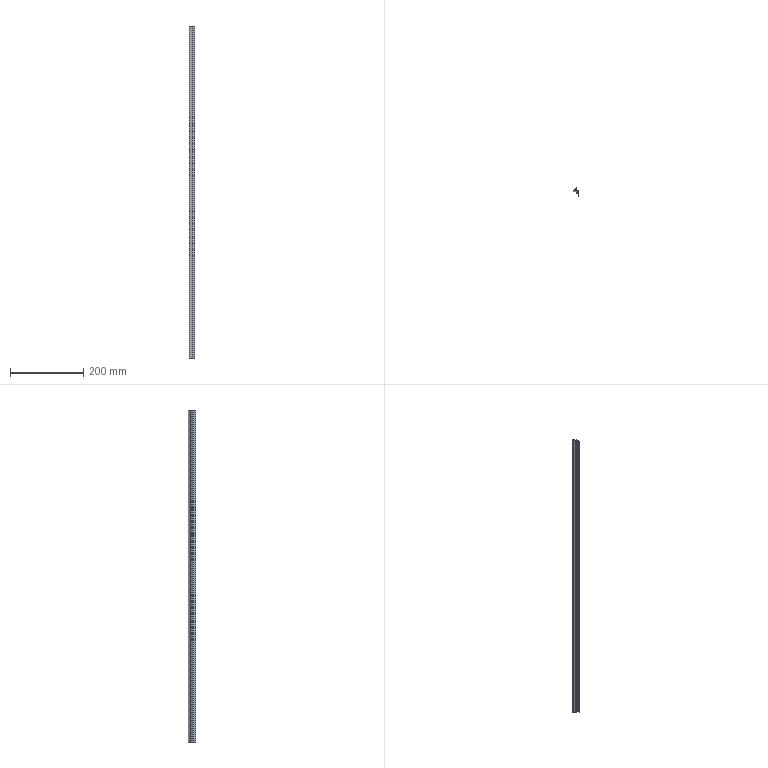Part | SolidWorks | features BaseBody 1, ICE 1, MoveFace 1 | 1 solid | 27 faces | box 14 x 20.3 x 907 mm | volume 46181 mm3 | plane 20 | cylinder 7 | commonest cylinder face diameters 0.387 x2 0.8 x2 0.4 x1 20 x1 22 x1
STEP:
#1=CARTESIAN_POINT('',(-5.304,-0.625,200.));
#2=VERTEX_POINT('',#1);
#3=CARTESIAN_POINT('',(-5.449,-0.8125,200.));
#4=VERTEX_POINT('',#3);
#5=CARTESIAN_POINT('',(-5.255,-0.8125,200.));
#6=DIRECTION('',(0.,0.,1.));
#7=DIRECTION('',(-1.,0.,0.));
#8=AXIS2_PLACEMENT_3D('',#5,#6,#7);
#9=CIRCLE('',#8,0.1937);
#10=EDGE_CURVE('',#2,#4,#9,.T.);
#11=ORIENTED_EDGE('',*,*,#10,.T.);
#12=CARTESIAN_POINT('',(-5.449,-0.8125,-707.));
#13=VERTEX_POINT('',#12);
#14=CARTESIAN_POINT('',(-5.449,-0.8125,230.));
#15=DIRECTION('',(0.,0.,-1.));
#16=VECTOR('',#15,1000.);
#17=LINE('',#14,#16);
#18=EDGE_CURVE('',#4,#13,#17,.T.);
#19=ORIENTED_EDGE('',*,*,#18,.T.);
#20=CARTESIAN_POINT('',(-5.304,-0.625,-707.));
#21=VERTEX_POINT('',#20);
#22=CARTESIAN_POINT('',(-5.255,-0.8125,-707.));
#23=DIRECTION('',(0.,0.,-1.));
#24=DIRECTION('',(1.,0.,0.));
#25=AXIS2_PLACEMENT_3D('',#22,#23,#24);
#26=CIRCLE('',#25,0.1937);
#27=EDGE_CURVE('',#13,#21,#26,.T.);
#28=ORIENTED_EDGE('',*,*,#27,.T.);
#29=CARTESIAN_POINT('',(-5.304,-0.625,230.));
#30=DIRECTION('',(0.,0.,-1.));
#31=VECTOR('',#30,1000.);
#32=LINE('',#29,#31);
#33=EDGE_CURVE('',#2,#21,#32,.T.);
#34=ORIENTED_EDGE('',*,*,#33,.F.);
#35=EDGE_LOOP('',(#11,#19,#28,#34));
#36=FACE_OUTER_BOUND('',#35,.T.);
#37=CARTESIAN_POINT('',(-5.255,-0.8125,230.));
#38=DIRECTION('',(0.,0.,-1.));
#39=DIRECTION('',(-1.,0.,0.));
#40=AXIS2_PLACEMENT_3D('',#37,#38,#39);
#41=CYLINDRICAL_SURFACE('',#40,0.1937);
#42=ADVANCED_FACE('',(#36),#41,.F.);
#43=CARTESIAN_POINT('',(5.,-1.,-707.));
#44=VERTEX_POINT('',#43);
#45=CARTESIAN_POINT('',(5.,-14.3,-707.));
#46=VERTEX_POINT('',#45);
#47=CARTESIAN_POINT('',(5.,29.623,-707.));
#48=DIRECTION('',(0.,-1.,0.));
#49=VECTOR('',#48,1000.);
#50=LINE('',#47,#49);
#51=EDGE_CURVE('',#44,#46,#50,.T.);
#52=ORIENTED_EDGE('',*,*,#51,.F.);
#53=CARTESIAN_POINT('',(5.,-1.,200.));
#54=VERTEX_POINT('',#53);
#55=CARTESIAN_POINT('',(5.,-1.,230.));
#56=DIRECTION('',(0.,0.,-1.));
#57=VECTOR('',#56,1000.);
#58=LINE('',#55,#57);
#59=EDGE_CURVE('',#54,#44,#58,.T.);
#60=ORIENTED_EDGE('',*,*,#59,.F.);
#61=CARTESIAN_POINT('',(5.,-14.3,200.));
#62=VERTEX_POINT('',#61);
#63=CARTESIAN_POINT('',(5.,-14.3,200.));
#64=DIRECTION('',(0.,1.,0.));
#65=VECTOR('',#64,1000.);
#66=LINE('',#63,#65);
#67=EDGE_CURVE('',#62,#54,#66,.T.);
#68=ORIENTED_EDGE('',*,*,#67,.F.);
#69=CARTESIAN_POINT('',(5.,-14.3,230.));
#70=DIRECTION('',(0.,0.,1.));
#71=VECTOR('',#70,1000.);
#72=LINE('',#69,#71);
#73=EDGE_CURVE('',#46,#62,#72,.T.);
#74=ORIENTED_EDGE('',*,*,#73,.F.);
#75=EDGE_LOOP('',(#52,#60,#68,#74));
#76=FACE_OUTER_BOUND('',#75,.T.);
#77=CARTESIAN_POINT('',(5.,-14.3,230.));
#78=DIRECTION('',(-1.,0.,0.));
#79=DIRECTION('',(0.,0.,1.));
#80=AXIS2_PLACEMENT_3D('',#77,#78,#79);
#81=PLANE('',#80);
#82=ADVANCED_FACE('',(#76),#81,.F.);
#83=CARTESIAN_POINT('',(-9.,-2.,-707.));
#84=VERTEX_POINT('',#83);
#85=CARTESIAN_POINT('',(-9.,-2.,200.));
#86=VERTEX_POINT('',#85);
#87=CARTESIAN_POINT('',(-9.,-2.,230.));
#88=DIRECTION('',(0.,0.,1.));
#89=VECTOR('',#88,1000.);
#90=LINE('',#87,#89);
#91=EDGE_CURVE('',#84,#86,#90,.T.);
#92=ORIENTED_EDGE('',*,*,#91,.F.);
#93=CARTESIAN_POINT('',(0.9,-2.,-707.));
#94=VERTEX_POINT('',#93);
#95=CARTESIAN_POINT('',(5.,-2.,-707.));
#96=DIRECTION('',(-1.,0.,0.));
#97=VECTOR('',#96,1000.);
#98=LINE('',#95,#97);
#99=EDGE_CURVE('',#94,#84,#98,.T.);
#100=ORIENTED_EDGE('',*,*,#99,.F.);
#101=CARTESIAN_POINT('',(0.9,-2.,200.));
#102=VERTEX_POINT('',#101);
#103=CARTESIAN_POINT('',(0.9,-2.,230.));
#104=DIRECTION('',(0.,0.,-1.));
#105=VECTOR('',#104,1000.);
#106=LINE('',#103,#105);
#107=EDGE_CURVE('',#102,#94,#106,.T.);
#108=ORIENTED_EDGE('',*,*,#107,.F.);
#109=CARTESIAN_POINT('',(5.,-2.,200.));
#110=DIRECTION('',(1.,0.,0.));
#111=VECTOR('',#110,1000.);
#112=LINE('',#109,#111);
#113=EDGE_CURVE('',#86,#102,#112,.T.);
#114=ORIENTED_EDGE('',*,*,#113,.F.);
#115=EDGE_LOOP('',(#92,#100,#108,#114));
#116=FACE_OUTER_BOUND('',#115,.T.);
#117=CARTESIAN_POINT('',(-9.,-2.,230.));
#118=DIRECTION('',(0.,1.,0.));
#119=DIRECTION('',(0.,0.,1.));
#120=AXIS2_PLACEMENT_3D('',#117,#118,#119);
#121=PLANE('',#120);
#122=ADVANCED_FACE('',(#116),#121,.F.);
#123=CARTESIAN_POINT('',(4.,-6.,200.));
#124=VERTEX_POINT('',#123);
#125=CARTESIAN_POINT('',(4.,-3.,200.));
#126=VERTEX_POINT('',#125);
#127=CARTESIAN_POINT('',(4.,29.623,200.));
#128=DIRECTION('',(0.,1.,0.));
#129=VECTOR('',#128,1000.);
#130=LINE('',#127,#129);
#131=EDGE_CURVE('',#124,#126,#130,.T.);
#132=ORIENTED_EDGE('',*,*,#131,.F.);
#133=CARTESIAN_POINT('',(1.,-6.,200.));
#134=VERTEX_POINT('',#133);
#135=CARTESIAN_POINT('',(5.,-6.,200.));
#136=DIRECTION('',(1.,0.,0.));
#137=VECTOR('',#136,1000.);
#138=LINE('',#135,#137);
#139=EDGE_CURVE('',#134,#124,#138,.T.);
#140=ORIENTED_EDGE('',*,*,#139,.F.);
#141=CARTESIAN_POINT('',(1.,-6.7,200.));
#142=VERTEX_POINT('',#141);
#143=CARTESIAN_POINT('',(1.,-6.,200.));
#144=DIRECTION('',(0.,-1.,0.));
#145=VECTOR('',#144,1000.);
#146=LINE('',#143,#145);
#147=EDGE_CURVE('',#134,#142,#146,.T.);
#148=ORIENTED_EDGE('',*,*,#147,.T.);
#149=CARTESIAN_POINT('',(-1.7,-6.7,200.));
#150=VERTEX_POINT('',#149);
#151=CARTESIAN_POINT('',(5.,-6.7,200.));
#152=DIRECTION('',(1.,0.,0.));
#153=VECTOR('',#152,1000.);
#154=LINE('',#151,#153);
#155=EDGE_CURVE('',#150,#142,#154,.T.);
#156=ORIENTED_EDGE('',*,*,#155,.F.);
#157=CARTESIAN_POINT('',(-1.7,-7.7,200.));
#158=VERTEX_POINT('',#157);
#159=CARTESIAN_POINT('',(-1.7,-6.7,200.));
#160=DIRECTION('',(0.,-1.,0.));
#161=VECTOR('',#160,1000.);
#162=LINE('',#159,#161);
#163=EDGE_CURVE('',#150,#158,#162,.T.);
#164=ORIENTED_EDGE('',*,*,#163,.T.);
#165=CARTESIAN_POINT('',(4.,-7.7,200.));
#166=VERTEX_POINT('',#165);
#167=CARTESIAN_POINT('',(5.,-7.7,200.));
#168=DIRECTION('',(-1.,0.,0.));
#169=VECTOR('',#168,1000.);
#170=LINE('',#167,#169);
#171=EDGE_CURVE('',#166,#158,#170,.T.);
#172=ORIENTED_EDGE('',*,*,#171,.F.);
#173=CARTESIAN_POINT('',(4.,-14.3,200.));
#174=VERTEX_POINT('',#173);
#175=CARTESIAN_POINT('',(4.,29.623,200.));
#176=DIRECTION('',(0.,1.,0.));
#177=VECTOR('',#176,1000.);
#178=LINE('',#175,#177);
#179=EDGE_CURVE('',#174,#166,#178,.T.);
#180=ORIENTED_EDGE('',*,*,#179,.F.);
#181=CARTESIAN_POINT('',(5.,-14.3,200.));
#182=DIRECTION('',(-1.,0.,0.));
#183=VECTOR('',#182,1000.);
#184=LINE('',#181,#183);
#185=EDGE_CURVE('',#62,#174,#184,.T.);
#186=ORIENTED_EDGE('',*,*,#185,.F.);
#187=ORIENTED_EDGE('',*,*,#67,.T.);
#188=CARTESIAN_POINT('',(-5.207,-1.,200.));
#189=VERTEX_POINT('',#188);
#190=CARTESIAN_POINT('',(5.,-1.,200.));
#191=DIRECTION('',(1.,0.,0.));
#192=VECTOR('',#191,1000.);
#193=LINE('',#190,#192);
#194=EDGE_CURVE('',#189,#54,#193,.T.);
#195=ORIENTED_EDGE('',*,*,#194,.F.);
#196=CARTESIAN_POINT('',(-5.255,-0.8125,200.));
#197=DIRECTION('',(0.,0.,1.));
#198=DIRECTION('',(-1.,0.,0.));
#199=AXIS2_PLACEMENT_3D('',#196,#197,#198);
#200=CIRCLE('',#199,0.1937);
#201=EDGE_CURVE('',#4,#189,#200,.T.);
#202=ORIENTED_EDGE('',*,*,#201,.F.);
#203=ORIENTED_EDGE('',*,*,#10,.F.);
#204=CARTESIAN_POINT('',(-1.368,3.063,200.));
#205=VERTEX_POINT('',#204);
#206=CARTESIAN_POINT('',(-10.628,9.,200.));
#207=DIRECTION('',(0.,0.,1.));
#208=DIRECTION('',(-1.,0.,0.));
#209=AXIS2_PLACEMENT_3D('',#206,#207,#208);
#210=CIRCLE('',#209,11.);
#211=EDGE_CURVE('',#2,#205,#210,.T.);
#212=ORIENTED_EDGE('',*,*,#211,.T.);
#213=CARTESIAN_POINT('',(-1.,2.955,200.));
#214=VERTEX_POINT('',#213);
#215=CARTESIAN_POINT('',(-1.2,2.955,200.));
#216=DIRECTION('',(0.,0.,1.));
#217=DIRECTION('',(-1.,0.,0.));
#218=AXIS2_PLACEMENT_3D('',#215,#216,#217);
#219=CIRCLE('',#218,0.2);
#220=EDGE_CURVE('',#214,#205,#219,.T.);
#221=ORIENTED_EDGE('',*,*,#220,.F.);
#222=CARTESIAN_POINT('',(-1.,1.5,200.));
#223=VERTEX_POINT('',#222);
#224=CARTESIAN_POINT('',(-1.,2.955,200.));
#225=DIRECTION('',(0.,1.,0.));
#226=VECTOR('',#225,1000.);
#227=LINE('',#224,#226);
#228=EDGE_CURVE('',#223,#214,#227,.T.);
#229=ORIENTED_EDGE('',*,*,#228,.F.);
#230=CARTESIAN_POINT('',(0.,1.5,200.));
#231=VERTEX_POINT('',#230);
#232=CARTESIAN_POINT('',(-1.,1.5,200.));
#233=DIRECTION('',(-1.,0.,0.));
#234=VECTOR('',#233,1000.);
#235=LINE('',#232,#234);
#236=EDGE_CURVE('',#231,#223,#235,.T.);
#237=ORIENTED_EDGE('',*,*,#236,.F.);
#238=CARTESIAN_POINT('',(0.,6.,200.));
#239=VERTEX_POINT('',#238);
#240=CARTESIAN_POINT('',(0.,1.5,200.));
#241=DIRECTION('',(0.,-1.,0.));
#242=VECTOR('',#241,1000.);
#243=LINE('',#240,#242);
#244=EDGE_CURVE('',#239,#231,#243,.T.);
#245=ORIENTED_EDGE('',*,*,#244,.F.);
#246=CARTESIAN_POINT('',(-0.8,6.,200.));
#247=VERTEX_POINT('',#246);
#248=CARTESIAN_POINT('',(0.,6.,200.));
#249=DIRECTION('',(1.,0.,0.));
#250=VECTOR('',#249,1000.);
#251=LINE('',#248,#250);
#252=EDGE_CURVE('',#247,#239,#251,.T.);
#253=ORIENTED_EDGE('',*,*,#252,.F.);
#254=CARTESIAN_POINT('',(-1.178,5.731,200.));
#255=VERTEX_POINT('',#254);
#256=CARTESIAN_POINT('',(-0.8,5.6,200.));
#257=DIRECTION('',(0.,0.,1.));
#258=DIRECTION('',(-1.,0.,0.));
#259=AXIS2_PLACEMENT_3D('',#256,#257,#258);
#260=CIRCLE('',#259,0.4);
#261=EDGE_CURVE('',#247,#255,#260,.T.);
#262=ORIENTED_EDGE('',*,*,#261,.T.);
#263=CARTESIAN_POINT('',(-8.678,-0.8077,200.));
#264=VERTEX_POINT('',#263);
#265=CARTESIAN_POINT('',(-10.628,9.,200.));
#266=DIRECTION('',(0.,0.,1.));
#267=DIRECTION('',(-1.,0.,0.));
#268=AXIS2_PLACEMENT_3D('',#265,#266,#267);
#269=CIRCLE('',#268,10.);
#270=EDGE_CURVE('',#264,#255,#269,.T.);
#271=ORIENTED_EDGE('',*,*,#270,.F.);
#272=CARTESIAN_POINT('',(-9.,-1.2,200.));
#273=VERTEX_POINT('',#272);
#274=CARTESIAN_POINT('',(-8.6,-1.2,200.));
#275=DIRECTION('',(0.,0.,1.));
#276=DIRECTION('',(-1.,0.,0.));
#277=AXIS2_PLACEMENT_3D('',#274,#275,#276);
#278=CIRCLE('',#277,0.4);
#279=EDGE_CURVE('',#264,#273,#278,.T.);
#280=ORIENTED_EDGE('',*,*,#279,.T.);
#281=CARTESIAN_POINT('',(-9.,8.,200.));
#282=DIRECTION('',(0.,-1.,0.));
#283=VECTOR('',#282,1000.);
#284=LINE('',#281,#283);
#285=EDGE_CURVE('',#273,#86,#284,.T.);
#286=ORIENTED_EDGE('',*,*,#285,.T.);
#287=ORIENTED_EDGE('',*,*,#113,.T.);
#288=CARTESIAN_POINT('',(0.9,-3.,200.));
#289=VERTEX_POINT('',#288);
#290=CARTESIAN_POINT('',(0.9,29.623,200.));
#291=DIRECTION('',(0.,1.,0.));
#292=VECTOR('',#291,1000.);
#293=LINE('',#290,#292);
#294=EDGE_CURVE('',#289,#102,#293,.T.);
#295=ORIENTED_EDGE('',*,*,#294,.F.);
#296=CARTESIAN_POINT('',(5.,-3.,200.));
#297=DIRECTION('',(-1.,0.,0.));
#298=VECTOR('',#297,1000.);
#299=LINE('',#296,#298);
#300=EDGE_CURVE('',#126,#289,#299,.T.);
#301=ORIENTED_EDGE('',*,*,#300,.F.);
#302=EDGE_LOOP('',(#132,#140,#148,#156,#164,#172,#180,#186,#187,#195,#202,#203,#212,#221,#229,#237,#245,#253,#262,#271,#280,#286,#287,#295,#301));
#303=FACE_OUTER_BOUND('',#302,.T.);
#304=CARTESIAN_POINT('',(5.,29.623,200.));
#305=DIRECTION('',(0.,0.,-1.));
#306=DIRECTION('',(-1.,0.,0.));
#307=AXIS2_PLACEMENT_3D('',#304,#305,#306);
#308=PLANE('',#307);
#309=ADVANCED_FACE('',(#303),#308,.F.);
#310=ORIENTED_EDGE('',*,*,#185,.T.);
#311=CARTESIAN_POINT('',(4.,-14.3,-707.));
#312=VERTEX_POINT('',#311);
#313=CARTESIAN_POINT('',(4.,-14.3,230.));
#314=DIRECTION('',(0.,0.,1.));
#315=VECTOR('',#314,1000.);
#316=LINE('',#313,#315);
#317=EDGE_CURVE('',#312,#174,#316,.T.);
#318=ORIENTED_EDGE('',*,*,#317,.F.);
#319=CARTESIAN_POINT('',(5.,-14.3,-707.));
#320=DIRECTION('',(-1.,0.,0.));
#321=VECTOR('',#320,1000.);
#322=LINE('',#319,#321);
#323=EDGE_CURVE('',#46,#312,#322,.T.);
#324=ORIENTED_EDGE('',*,*,#323,.F.);
#325=ORIENTED_EDGE('',*,*,#73,.T.);
#326=EDGE_LOOP('',(#310,#318,#324,#325));
#327=FACE_OUTER_BOUND('',#326,.T.);
#328=CARTESIAN_POINT('',(4.,-14.3,230.));
#329=DIRECTION('',(0.,1.,0.));
#330=DIRECTION('',(0.,0.,1.));
#331=AXIS2_PLACEMENT_3D('',#328,#329,#330);
#332=PLANE('',#331);
#333=ADVANCED_FACE('',(#327),#332,.F.);
#334=ORIENTED_EDGE('',*,*,#51,.T.);
#335=ORIENTED_EDGE('',*,*,#323,.T.);
#336=CARTESIAN_POINT('',(4.,-7.7,-707.));
#337=VERTEX_POINT('',#336);
#338=CARTESIAN_POINT('',(4.,-7.7,-707.));
#339=DIRECTION('',(0.,-1.,0.));
#340=VECTOR('',#339,1000.);
#341=LINE('',#338,#340);
#342=EDGE_CURVE('',#337,#312,#341,.T.);
#343=ORIENTED_EDGE('',*,*,#342,.F.);
#344=CARTESIAN_POINT('',(-1.7,-7.7,-707.));
#345=VERTEX_POINT('',#344);
#346=CARTESIAN_POINT('',(-1.7,-7.7,-707.));
#347=DIRECTION('',(1.,0.,0.));
#348=VECTOR('',#347,1000.);
#349=LINE('',#346,#348);
#350=EDGE_CURVE('',#345,#337,#349,.T.);
#351=ORIENTED_EDGE('',*,*,#350,.F.);
#352=CARTESIAN_POINT('',(-1.7,-6.7,-707.));
#353=VERTEX_POINT('',#352);
#354=CARTESIAN_POINT('',(-1.7,29.623,-707.));
#355=DIRECTION('',(0.,1.,0.));
#356=VECTOR('',#355,1000.);
#357=LINE('',#354,#356);
#358=EDGE_CURVE('',#345,#353,#357,.T.);
#359=ORIENTED_EDGE('',*,*,#358,.T.);
#360=CARTESIAN_POINT('',(1.,-6.7,-707.));
#361=VERTEX_POINT('',#360);
#362=CARTESIAN_POINT('',(1.,-6.7,-707.));
#363=DIRECTION('',(-1.,0.,0.));
#364=VECTOR('',#363,1000.);
#365=LINE('',#362,#364);
#366=EDGE_CURVE('',#361,#353,#365,.T.);
#367=ORIENTED_EDGE('',*,*,#366,.F.);
#368=CARTESIAN_POINT('',(1.,-6.,-707.));
#369=VERTEX_POINT('',#368);
#370=CARTESIAN_POINT('',(1.,29.623,-707.));
#371=DIRECTION('',(0.,1.,0.));
#372=VECTOR('',#371,1000.);
#373=LINE('',#370,#372);
#374=EDGE_CURVE('',#361,#369,#373,.T.);
#375=ORIENTED_EDGE('',*,*,#374,.T.);
#376=CARTESIAN_POINT('',(4.,-6.,-707.));
#377=VERTEX_POINT('',#376);
#378=CARTESIAN_POINT('',(4.,-6.,-707.));
#379=DIRECTION('',(-1.,0.,0.));
#380=VECTOR('',#379,1000.);
#381=LINE('',#378,#380);
#382=EDGE_CURVE('',#377,#369,#381,.T.);
#383=ORIENTED_EDGE('',*,*,#382,.F.);
#384=CARTESIAN_POINT('',(4.,-3.,-707.));
#385=VERTEX_POINT('',#384);
#386=CARTESIAN_POINT('',(4.,-3.,-707.));
#387=DIRECTION('',(0.,-1.,0.));
#388=VECTOR('',#387,1000.);
#389=LINE('',#386,#388);
#390=EDGE_CURVE('',#385,#377,#389,.T.);
#391=ORIENTED_EDGE('',*,*,#390,.F.);
#392=CARTESIAN_POINT('',(0.9,-3.,-707.));
#393=VERTEX_POINT('',#392);
#394=CARTESIAN_POINT('',(0.9,-3.,-707.));
#395=DIRECTION('',(1.,0.,0.));
#396=VECTOR('',#395,1000.);
#397=LINE('',#394,#396);
#398=EDGE_CURVE('',#393,#385,#397,.T.);
#399=ORIENTED_EDGE('',*,*,#398,.F.);
#400=CARTESIAN_POINT('',(0.9,-2.,-707.));
#401=DIRECTION('',(0.,-1.,0.));
#402=VECTOR('',#401,1000.);
#403=LINE('',#400,#402);
#404=EDGE_CURVE('',#94,#393,#403,.T.);
#405=ORIENTED_EDGE('',*,*,#404,.F.);
#406=ORIENTED_EDGE('',*,*,#99,.T.);
#407=CARTESIAN_POINT('',(-9.,-1.2,-707.));
#408=VERTEX_POINT('',#407);
#409=CARTESIAN_POINT('',(-9.,-1.2,-707.));
#410=DIRECTION('',(0.,-1.,0.));
#411=VECTOR('',#410,1000.);
#412=LINE('',#409,#411);
#413=EDGE_CURVE('',#408,#84,#412,.T.);
#414=ORIENTED_EDGE('',*,*,#413,.F.);
#415=CARTESIAN_POINT('',(-8.678,-0.8077,-707.));
#416=VERTEX_POINT('',#415);
#417=CARTESIAN_POINT('',(-8.6,-1.2,-707.));
#418=DIRECTION('',(0.,0.,-1.));
#419=DIRECTION('',(1.,0.,0.));
#420=AXIS2_PLACEMENT_3D('',#417,#418,#419);
#421=CIRCLE('',#420,0.4);
#422=EDGE_CURVE('',#408,#416,#421,.T.);
#423=ORIENTED_EDGE('',*,*,#422,.T.);
#424=CARTESIAN_POINT('',(-1.178,5.731,-707.));
#425=VERTEX_POINT('',#424);
#426=CARTESIAN_POINT('',(-10.628,9.,-707.));
#427=DIRECTION('',(0.,0.,-1.));
#428=DIRECTION('',(1.,0.,0.));
#429=AXIS2_PLACEMENT_3D('',#426,#427,#428);
#430=CIRCLE('',#429,10.);
#431=EDGE_CURVE('',#425,#416,#430,.T.);
#432=ORIENTED_EDGE('',*,*,#431,.F.);
#433=CARTESIAN_POINT('',(-0.8,6.,-707.));
#434=VERTEX_POINT('',#433);
#435=CARTESIAN_POINT('',(-0.8,5.6,-707.));
#436=DIRECTION('',(0.,0.,-1.));
#437=DIRECTION('',(1.,0.,0.));
#438=AXIS2_PLACEMENT_3D('',#435,#436,#437);
#439=CIRCLE('',#438,0.4);
#440=EDGE_CURVE('',#425,#434,#439,.T.);
#441=ORIENTED_EDGE('',*,*,#440,.T.);
#442=CARTESIAN_POINT('',(0.,6.,-707.));
#443=VERTEX_POINT('',#442);
#444=CARTESIAN_POINT('',(0.,6.,-707.));
#445=DIRECTION('',(-1.,0.,0.));
#446=VECTOR('',#445,1000.);
#447=LINE('',#444,#446);
#448=EDGE_CURVE('',#443,#434,#447,.T.);
#449=ORIENTED_EDGE('',*,*,#448,.F.);
#450=CARTESIAN_POINT('',(0.,1.5,-707.));
#451=VERTEX_POINT('',#450);
#452=CARTESIAN_POINT('',(0.,1.5,-707.));
#453=DIRECTION('',(0.,1.,0.));
#454=VECTOR('',#453,1000.);
#455=LINE('',#452,#454);
#456=EDGE_CURVE('',#451,#443,#455,.T.);
#457=ORIENTED_EDGE('',*,*,#456,.F.);
#458=CARTESIAN_POINT('',(-1.,1.5,-707.));
#459=VERTEX_POINT('',#458);
#460=CARTESIAN_POINT('',(-1.,1.5,-707.));
#461=DIRECTION('',(1.,0.,0.));
#462=VECTOR('',#461,1000.);
#463=LINE('',#460,#462);
#464=EDGE_CURVE('',#459,#451,#463,.T.);
#465=ORIENTED_EDGE('',*,*,#464,.F.);
#466=CARTESIAN_POINT('',(-1.,2.955,-707.));
#467=VERTEX_POINT('',#466);
#468=CARTESIAN_POINT('',(-1.,2.955,-707.));
#469=DIRECTION('',(0.,-1.,0.));
#470=VECTOR('',#469,1000.);
#471=LINE('',#468,#470);
#472=EDGE_CURVE('',#467,#459,#471,.T.);
#473=ORIENTED_EDGE('',*,*,#472,.F.);
#474=CARTESIAN_POINT('',(-1.368,3.063,-707.));
#475=VERTEX_POINT('',#474);
#476=CARTESIAN_POINT('',(-1.2,2.955,-707.));
#477=DIRECTION('',(0.,0.,-1.));
#478=DIRECTION('',(1.,0.,0.));
#479=AXIS2_PLACEMENT_3D('',#476,#477,#478);
#480=CIRCLE('',#479,0.2);
#481=EDGE_CURVE('',#475,#467,#480,.T.);
#482=ORIENTED_EDGE('',*,*,#481,.F.);
#483=CARTESIAN_POINT('',(-10.628,9.,-707.));
#484=DIRECTION('',(0.,0.,-1.));
#485=DIRECTION('',(1.,0.,0.));
#486=AXIS2_PLACEMENT_3D('',#483,#484,#485);
#487=CIRCLE('',#486,11.);
#488=EDGE_CURVE('',#475,#21,#487,.T.);
#489=ORIENTED_EDGE('',*,*,#488,.T.);
#490=ORIENTED_EDGE('',*,*,#27,.F.);
#491=CARTESIAN_POINT('',(-5.207,-1.,-707.));
#492=VERTEX_POINT('',#491);
#493=CARTESIAN_POINT('',(-5.255,-0.8125,-707.));
#494=DIRECTION('',(0.,0.,-1.));
#495=DIRECTION('',(1.,0.,0.));
#496=AXIS2_PLACEMENT_3D('',#493,#494,#495);
#497=CIRCLE('',#496,0.1937);
#498=EDGE_CURVE('',#492,#13,#497,.T.);
#499=ORIENTED_EDGE('',*,*,#498,.F.);
#500=CARTESIAN_POINT('',(5.,-1.,-707.));
#501=DIRECTION('',(-1.,0.,0.));
#502=VECTOR('',#501,1000.);
#503=LINE('',#500,#502);
#504=EDGE_CURVE('',#44,#492,#503,.T.);
#505=ORIENTED_EDGE('',*,*,#504,.F.);
#506=EDGE_LOOP('',(#334,#335,#343,#351,#359,#367,#375,#383,#391,#399,#405,#406,#414,#423,#432,#441,#449,#457,#465,#473,#482,#489,#490,#499,#505));
#507=FACE_OUTER_BOUND('',#506,.T.);
#508=CARTESIAN_POINT('',(5.,29.623,-707.));
#509=DIRECTION('',(0.,0.,1.));
#510=DIRECTION('',(1.,0.,0.));
#511=AXIS2_PLACEMENT_3D('',#508,#509,#510);
#512=PLANE('',#511);
#513=ADVANCED_FACE('',(#507),#512,.F.);
#514=ORIENTED_EDGE('',*,*,#59,.T.);
#515=ORIENTED_EDGE('',*,*,#504,.T.);
#516=CARTESIAN_POINT('',(-5.207,-1.,230.));
#517=DIRECTION('',(0.,0.,-1.));
#518=VECTOR('',#517,1000.);
#519=LINE('',#516,#518);
#520=EDGE_CURVE('',#189,#492,#519,.T.);
#521=ORIENTED_EDGE('',*,*,#520,.F.);
#522=ORIENTED_EDGE('',*,*,#194,.T.);
#523=EDGE_LOOP('',(#514,#515,#521,#522));
#524=FACE_OUTER_BOUND('',#523,.T.);
#525=CARTESIAN_POINT('',(5.,-1.,230.));
#526=DIRECTION('',(0.,-1.,0.));
#527=DIRECTION('',(0.,0.,-1.));
#528=AXIS2_PLACEMENT_3D('',#525,#526,#527);
#529=PLANE('',#528);
#530=ADVANCED_FACE('',(#524),#529,.F.);
#531=CARTESIAN_POINT('',(-9.,-1.2,230.));
#532=DIRECTION('',(0.,0.,1.));
#533=VECTOR('',#532,1000.);
#534=LINE('',#531,#533);
#535=EDGE_CURVE('',#408,#273,#534,.T.);
#536=ORIENTED_EDGE('',*,*,#535,.F.);
#537=ORIENTED_EDGE('',*,*,#413,.T.);
#538=ORIENTED_EDGE('',*,*,#91,.T.);
#539=ORIENTED_EDGE('',*,*,#285,.F.);
#540=EDGE_LOOP('',(#536,#537,#538,#539));
#541=FACE_OUTER_BOUND('',#540,.T.);
#542=CARTESIAN_POINT('',(-9.,-1.2,230.));
#543=DIRECTION('',(1.,0.,0.));
#544=DIRECTION('',(0.,0.,-1.));
#545=AXIS2_PLACEMENT_3D('',#542,#543,#544);
#546=PLANE('',#545);
#547=ADVANCED_FACE('',(#541),#546,.F.);
#548=ORIENTED_EDGE('',*,*,#294,.T.);
#549=ORIENTED_EDGE('',*,*,#107,.T.);
#550=ORIENTED_EDGE('',*,*,#404,.T.);
#551=CARTESIAN_POINT('',(0.9,-3.,230.));
#552=DIRECTION('',(0.,0.,-1.));
#553=VECTOR('',#552,1000.);
#554=LINE('',#551,#553);
#555=EDGE_CURVE('',#289,#393,#554,.T.);
#556=ORIENTED_EDGE('',*,*,#555,.F.);
#557=EDGE_LOOP('',(#548,#549,#550,#556));
#558=FACE_OUTER_BOUND('',#557,.T.);
#559=CARTESIAN_POINT('',(0.9,-2.,230.));
#560=DIRECTION('',(1.,0.,0.));
#561=DIRECTION('',(0.,0.,-1.));
#562=AXIS2_PLACEMENT_3D('',#559,#560,#561);
#563=PLANE('',#562);
#564=ADVANCED_FACE('',(#558),#563,.F.);
#565=ORIENTED_EDGE('',*,*,#300,.T.);
#566=ORIENTED_EDGE('',*,*,#555,.T.);
#567=ORIENTED_EDGE('',*,*,#398,.T.);
#568=CARTESIAN_POINT('',(4.,-3.,230.));
#569=DIRECTION('',(0.,0.,-1.));
#570=VECTOR('',#569,1000.);
#571=LINE('',#568,#570);
#572=EDGE_CURVE('',#126,#385,#571,.T.);
#573=ORIENTED_EDGE('',*,*,#572,.F.);
#574=EDGE_LOOP('',(#565,#566,#567,#573));
#575=FACE_OUTER_BOUND('',#574,.T.);
#576=CARTESIAN_POINT('',(0.9,-3.,230.));
#577=DIRECTION('',(0.,1.,0.));
#578=DIRECTION('',(0.,0.,1.));
#579=AXIS2_PLACEMENT_3D('',#576,#577,#578);
#580=PLANE('',#579);
#581=ADVANCED_FACE('',(#575),#580,.F.);
#582=ORIENTED_EDGE('',*,*,#131,.T.);
#583=ORIENTED_EDGE('',*,*,#572,.T.);
#584=ORIENTED_EDGE('',*,*,#390,.T.);
#585=CARTESIAN_POINT('',(4.,-6.,230.));
#586=DIRECTION('',(0.,0.,-1.));
#587=VECTOR('',#586,1000.);
#588=LINE('',#585,#587);
#589=EDGE_CURVE('',#124,#377,#588,.T.);
#590=ORIENTED_EDGE('',*,*,#589,.F.);
#591=EDGE_LOOP('',(#582,#583,#584,#590));
#592=FACE_OUTER_BOUND('',#591,.T.);
#593=CARTESIAN_POINT('',(4.,-3.,230.));
#594=DIRECTION('',(1.,0.,0.));
#595=DIRECTION('',(0.,0.,-1.));
#596=AXIS2_PLACEMENT_3D('',#593,#594,#595);
#597=PLANE('',#596);
#598=ADVANCED_FACE('',(#592),#597,.F.);
#599=ORIENTED_EDGE('',*,*,#139,.T.);
#600=ORIENTED_EDGE('',*,*,#589,.T.);
#601=ORIENTED_EDGE('',*,*,#382,.T.);
#602=CARTESIAN_POINT('',(1.,-6.,230.));
#603=DIRECTION('',(0.,0.,-1.));
#604=VECTOR('',#603,1000.);
#605=LINE('',#602,#604);
#606=EDGE_CURVE('',#134,#369,#605,.T.);
#607=ORIENTED_EDGE('',*,*,#606,.F.);
#608=EDGE_LOOP('',(#599,#600,#601,#607));
#609=FACE_OUTER_BOUND('',#608,.T.);
#610=CARTESIAN_POINT('',(4.,-6.,230.));
#611=DIRECTION('',(0.,-1.,0.));
#612=DIRECTION('',(0.,0.,-1.));
#613=AXIS2_PLACEMENT_3D('',#610,#611,#612);
#614=PLANE('',#613);
#615=ADVANCED_FACE('',(#609),#614,.F.);
#616=ORIENTED_EDGE('',*,*,#155,.T.);
#617=CARTESIAN_POINT('',(1.,-6.7,230.));
#618=DIRECTION('',(0.,0.,1.));
#619=VECTOR('',#618,1000.);
#620=LINE('',#617,#619);
#621=EDGE_CURVE('',#361,#142,#620,.T.);
#622=ORIENTED_EDGE('',*,*,#621,.F.);
#623=ORIENTED_EDGE('',*,*,#366,.T.);
#624=CARTESIAN_POINT('',(-1.7,-6.7,230.));
#625=DIRECTION('',(0.,0.,-1.));
#626=VECTOR('',#625,1000.);
#627=LINE('',#624,#626);
#628=EDGE_CURVE('',#150,#353,#627,.T.);
#629=ORIENTED_EDGE('',*,*,#628,.F.);
#630=EDGE_LOOP('',(#616,#622,#623,#629));
#631=FACE_OUTER_BOUND('',#630,.T.);
#632=CARTESIAN_POINT('',(1.,-6.7,230.));
#633=DIRECTION('',(0.,-1.,0.));
#634=DIRECTION('',(0.,0.,-1.));
#635=AXIS2_PLACEMENT_3D('',#632,#633,#634);
#636=PLANE('',#635);
#637=ADVANCED_FACE('',(#631),#636,.F.);
#638=ORIENTED_EDGE('',*,*,#171,.T.);
#639=CARTESIAN_POINT('',(-1.7,-7.7,230.));
#640=DIRECTION('',(0.,0.,1.));
#641=VECTOR('',#640,1000.);
#642=LINE('',#639,#641);
#643=EDGE_CURVE('',#345,#158,#642,.T.);
#644=ORIENTED_EDGE('',*,*,#643,.F.);
#645=ORIENTED_EDGE('',*,*,#350,.T.);
#646=CARTESIAN_POINT('',(4.,-7.7,230.));
#647=DIRECTION('',(0.,0.,-1.));
#648=VECTOR('',#647,1000.);
#649=LINE('',#646,#648);
#650=EDGE_CURVE('',#166,#337,#649,.T.);
#651=ORIENTED_EDGE('',*,*,#650,.F.);
#652=EDGE_LOOP('',(#638,#644,#645,#651));
#653=FACE_OUTER_BOUND('',#652,.T.);
#654=CARTESIAN_POINT('',(-1.7,-7.7,230.));
#655=DIRECTION('',(0.,1.,0.));
#656=DIRECTION('',(0.,0.,1.));
#657=AXIS2_PLACEMENT_3D('',#654,#655,#656);
#658=PLANE('',#657);
#659=ADVANCED_FACE('',(#653),#658,.F.);
#660=ORIENTED_EDGE('',*,*,#179,.T.);
#661=ORIENTED_EDGE('',*,*,#650,.T.);
#662=ORIENTED_EDGE('',*,*,#342,.T.);
#663=ORIENTED_EDGE('',*,*,#317,.T.);
#664=EDGE_LOOP('',(#660,#661,#662,#663));
#665=FACE_OUTER_BOUND('',#664,.T.);
#666=CARTESIAN_POINT('',(4.,-7.7,230.));
#667=DIRECTION('',(1.,0.,0.));
#668=DIRECTION('',(0.,0.,-1.));
#669=AXIS2_PLACEMENT_3D('',#666,#667,#668);
#670=PLANE('',#669);
#671=ADVANCED_FACE('',(#665),#670,.F.);
#672=ORIENTED_EDGE('',*,*,#18,.F.);
#673=ORIENTED_EDGE('',*,*,#201,.T.);
#674=ORIENTED_EDGE('',*,*,#520,.T.);
#675=ORIENTED_EDGE('',*,*,#498,.T.);
#676=EDGE_LOOP('',(#672,#673,#674,#675));
#677=FACE_OUTER_BOUND('',#676,.T.);
#678=CARTESIAN_POINT('',(-5.255,-0.8125,230.));
#679=DIRECTION('',(0.,0.,-1.));
#680=DIRECTION('',(-1.,0.,0.));
#681=AXIS2_PLACEMENT_3D('',#678,#679,#680);
#682=CYLINDRICAL_SURFACE('',#681,0.1937);
#683=ADVANCED_FACE('',(#677),#682,.F.);
#684=CARTESIAN_POINT('',(-1.,2.955,230.));
#685=DIRECTION('',(0.,0.,1.));
#686=VECTOR('',#685,1000.);
#687=LINE('',#684,#686);
#688=EDGE_CURVE('',#467,#214,#687,.T.);
#689=ORIENTED_EDGE('',*,*,#688,.F.);
#690=ORIENTED_EDGE('',*,*,#472,.T.);
#691=CARTESIAN_POINT('',(-1.,1.5,230.));
#692=DIRECTION('',(0.,0.,-1.));
#693=VECTOR('',#692,1000.);
#694=LINE('',#691,#693);
#695=EDGE_CURVE('',#223,#459,#694,.T.);
#696=ORIENTED_EDGE('',*,*,#695,.F.);
#697=ORIENTED_EDGE('',*,*,#228,.T.);
#698=EDGE_LOOP('',(#689,#690,#696,#697));
#699=FACE_OUTER_BOUND('',#698,.T.);
#700=CARTESIAN_POINT('',(-1.,2.955,230.));
#701=DIRECTION('',(1.,0.,0.));
#702=DIRECTION('',(0.,0.,-1.));
#703=AXIS2_PLACEMENT_3D('',#700,#701,#702);
#704=PLANE('',#703);
#705=ADVANCED_FACE('',(#699),#704,.F.);
#706=ORIENTED_EDGE('',*,*,#488,.F.);
#707=CARTESIAN_POINT('',(-1.368,3.063,230.));
#708=DIRECTION('',(0.,0.,1.));
#709=VECTOR('',#708,1000.);
#710=LINE('',#707,#709);
#711=EDGE_CURVE('',#475,#205,#710,.T.);
#712=ORIENTED_EDGE('',*,*,#711,.T.);
#713=ORIENTED_EDGE('',*,*,#211,.F.);
#714=ORIENTED_EDGE('',*,*,#33,.T.);
#715=EDGE_LOOP('',(#706,#712,#713,#714));
#716=FACE_OUTER_BOUND('',#715,.T.);
#717=CARTESIAN_POINT('',(-10.628,9.,230.));
#718=DIRECTION('',(0.,0.,-1.));
#719=DIRECTION('',(-1.,0.,0.));
#720=AXIS2_PLACEMENT_3D('',#717,#718,#719);
#721=CYLINDRICAL_SURFACE('',#720,11.);
#722=ADVANCED_FACE('',(#716),#721,.T.);
#723=CARTESIAN_POINT('',(-1.178,5.731,230.));
#724=DIRECTION('',(0.,0.,1.));
#725=VECTOR('',#724,1000.);
#726=LINE('',#723,#725);
#727=EDGE_CURVE('',#425,#255,#726,.T.);
#728=ORIENTED_EDGE('',*,*,#727,.F.);
#729=ORIENTED_EDGE('',*,*,#431,.T.);
#730=CARTESIAN_POINT('',(-8.678,-0.8077,230.));
#731=DIRECTION('',(0.,0.,-1.));
#732=VECTOR('',#731,1000.);
#733=LINE('',#730,#732);
#734=EDGE_CURVE('',#264,#416,#733,.T.);
#735=ORIENTED_EDGE('',*,*,#734,.F.);
#736=ORIENTED_EDGE('',*,*,#270,.T.);
#737=EDGE_LOOP('',(#728,#729,#735,#736));
#738=FACE_OUTER_BOUND('',#737,.T.);
#739=CARTESIAN_POINT('',(-10.628,9.,230.));
#740=DIRECTION('',(0.,0.,-1.));
#741=DIRECTION('',(-1.,0.,0.));
#742=AXIS2_PLACEMENT_3D('',#739,#740,#741);
#743=CYLINDRICAL_SURFACE('',#742,10.);
#744=ADVANCED_FACE('',(#738),#743,.F.);
#745=CARTESIAN_POINT('',(0.,1.5,230.));
#746=DIRECTION('',(0.,0.,1.));
#747=VECTOR('',#746,1000.);
#748=LINE('',#745,#747);
#749=EDGE_CURVE('',#451,#231,#748,.T.);
#750=ORIENTED_EDGE('',*,*,#749,.F.);
#751=ORIENTED_EDGE('',*,*,#456,.T.);
#752=CARTESIAN_POINT('',(0.,6.,230.));
#753=DIRECTION('',(0.,0.,-1.));
#754=VECTOR('',#753,1000.);
#755=LINE('',#752,#754);
#756=EDGE_CURVE('',#239,#443,#755,.T.);
#757=ORIENTED_EDGE('',*,*,#756,.F.);
#758=ORIENTED_EDGE('',*,*,#244,.T.);
#759=EDGE_LOOP('',(#750,#751,#757,#758));
#760=FACE_OUTER_BOUND('',#759,.T.);
#761=CARTESIAN_POINT('',(0.,1.5,230.));
#762=DIRECTION('',(-1.,0.,0.));
#763=DIRECTION('',(0.,0.,1.));
#764=AXIS2_PLACEMENT_3D('',#761,#762,#763);
#765=PLANE('',#764);
#766=ADVANCED_FACE('',(#760),#765,.F.);
#767=ORIENTED_EDGE('',*,*,#422,.F.);
#768=ORIENTED_EDGE('',*,*,#535,.T.);
#769=ORIENTED_EDGE('',*,*,#279,.F.);
#770=ORIENTED_EDGE('',*,*,#734,.T.);
#771=EDGE_LOOP('',(#767,#768,#769,#770));
#772=FACE_OUTER_BOUND('',#771,.T.);
#773=CARTESIAN_POINT('',(-8.6,-1.2,230.));
#774=DIRECTION('',(0.,0.,-1.));
#775=DIRECTION('',(-1.,0.,0.));
#776=AXIS2_PLACEMENT_3D('',#773,#774,#775);
#777=CYLINDRICAL_SURFACE('',#776,0.4);
#778=ADVANCED_FACE('',(#772),#777,.T.);
#779=ORIENTED_EDGE('',*,*,#147,.F.);
#780=ORIENTED_EDGE('',*,*,#606,.T.);
#781=ORIENTED_EDGE('',*,*,#374,.F.);
#782=ORIENTED_EDGE('',*,*,#621,.T.);
#783=EDGE_LOOP('',(#779,#780,#781,#782));
#784=FACE_OUTER_BOUND('',#783,.T.);
#785=CARTESIAN_POINT('',(1.,-6.,230.));
#786=DIRECTION('',(1.,0.,0.));
#787=DIRECTION('',(0.,0.,-1.));
#788=AXIS2_PLACEMENT_3D('',#785,#786,#787);
#789=PLANE('',#788);
#790=ADVANCED_FACE('',(#784),#789,.F.);
#791=ORIENTED_EDGE('',*,*,#163,.F.);
#792=ORIENTED_EDGE('',*,*,#628,.T.);
#793=ORIENTED_EDGE('',*,*,#358,.F.);
#794=ORIENTED_EDGE('',*,*,#643,.T.);
#795=EDGE_LOOP('',(#791,#792,#793,#794));
#796=FACE_OUTER_BOUND('',#795,.T.);
#797=CARTESIAN_POINT('',(-1.7,-6.7,230.));
#798=DIRECTION('',(1.,0.,0.));
#799=DIRECTION('',(0.,0.,-1.));
#800=AXIS2_PLACEMENT_3D('',#797,#798,#799);
#801=PLANE('',#800);
#802=ADVANCED_FACE('',(#796),#801,.F.);
#803=ORIENTED_EDGE('',*,*,#711,.F.);
#804=ORIENTED_EDGE('',*,*,#481,.T.);
#805=ORIENTED_EDGE('',*,*,#688,.T.);
#806=ORIENTED_EDGE('',*,*,#220,.T.);
#807=EDGE_LOOP('',(#803,#804,#805,#806));
#808=FACE_OUTER_BOUND('',#807,.T.);
#809=CARTESIAN_POINT('',(-1.2,2.955,230.));
#810=DIRECTION('',(0.,0.,-1.));
#811=DIRECTION('',(-1.,0.,0.));
#812=AXIS2_PLACEMENT_3D('',#809,#810,#811);
#813=CYLINDRICAL_SURFACE('',#812,0.2);
#814=ADVANCED_FACE('',(#808),#813,.F.);
#815=ORIENTED_EDGE('',*,*,#695,.T.);
#816=ORIENTED_EDGE('',*,*,#464,.T.);
#817=ORIENTED_EDGE('',*,*,#749,.T.);
#818=ORIENTED_EDGE('',*,*,#236,.T.);
#819=EDGE_LOOP('',(#815,#816,#817,#818));
#820=FACE_OUTER_BOUND('',#819,.T.);
#821=CARTESIAN_POINT('',(-1.,1.5,230.));
#822=DIRECTION('',(0.,1.,0.));
#823=DIRECTION('',(0.,0.,1.));
#824=AXIS2_PLACEMENT_3D('',#821,#822,#823);
#825=PLANE('',#824);
#826=ADVANCED_FACE('',(#820),#825,.F.);
#827=ORIENTED_EDGE('',*,*,#440,.F.);
#828=ORIENTED_EDGE('',*,*,#727,.T.);
#829=ORIENTED_EDGE('',*,*,#261,.F.);
#830=CARTESIAN_POINT('',(-0.8,6.,230.));
#831=DIRECTION('',(0.,0.,-1.));
#832=VECTOR('',#831,1000.);
#833=LINE('',#830,#832);
#834=EDGE_CURVE('',#247,#434,#833,.T.);
#835=ORIENTED_EDGE('',*,*,#834,.T.);
#836=EDGE_LOOP('',(#827,#828,#829,#835));
#837=FACE_OUTER_BOUND('',#836,.T.);
#838=CARTESIAN_POINT('',(-0.8,5.6,230.));
#839=DIRECTION('',(0.,0.,-1.));
#840=DIRECTION('',(-1.,0.,0.));
#841=AXIS2_PLACEMENT_3D('',#838,#839,#840);
#842=CYLINDRICAL_SURFACE('',#841,0.4);
#843=ADVANCED_FACE('',(#837),#842,.T.);
#844=ORIENTED_EDGE('',*,*,#756,.T.);
#845=ORIENTED_EDGE('',*,*,#448,.T.);
#846=ORIENTED_EDGE('',*,*,#834,.F.);
#847=ORIENTED_EDGE('',*,*,#252,.T.);
#848=EDGE_LOOP('',(#844,#845,#846,#847));
#849=FACE_OUTER_BOUND('',#848,.T.);
#850=CARTESIAN_POINT('',(0.,6.,230.));
#851=DIRECTION('',(0.,-1.,0.));
#852=DIRECTION('',(0.,0.,-1.));
#853=AXIS2_PLACEMENT_3D('',#850,#851,#852);
#854=PLANE('',#853);
#855=ADVANCED_FACE('',(#849),#854,.F.);
#856=CLOSED_SHELL('',(#42,#82,#122,#309,#333,#513,#530,#547,#564,#581,#598,#615,#637,#659,#671,#683,#705,#722,#744,#766,#778,#790,#802,#814,#826,#843,#855));
#857=MANIFOLD_SOLID_BREP('',#856);
#858=CARTESIAN_POINT('',(0.,0.,0.));
#859=DIRECTION('',(0.,0.,1.));
#860=DIRECTION('',(1.,0.,0.));
#861=AXIS2_PLACEMENT_3D('',#858,#859,#860);
#862=(LENGTH_UNIT()NAMED_UNIT(*)SI_UNIT(.MILLI.,.METRE.));
#863=UNCERTAINTY_MEASURE_WITH_UNIT(LENGTH_MEASURE(0.00001),#862,'','');
#864=(NAMED_UNIT(*)PLANE_ANGLE_UNIT()SI_UNIT($,.RADIAN.));
#865=(NAMED_UNIT(*)SI_UNIT($,.STERADIAN.)SOLID_ANGLE_UNIT());
#866=(GEOMETRIC_REPRESENTATION_CONTEXT(3)GLOBAL_UNCERTAINTY_ASSIGNED_CONTEXT((#863))GLOBAL_UNIT_ASSIGNED_CONTEXT((#862,#864,#865))REPRESENTATION_CONTEXT('',''));
#867=ADVANCED_BREP_SHAPE_REPRESENTATION('',(#857,#861),#866);